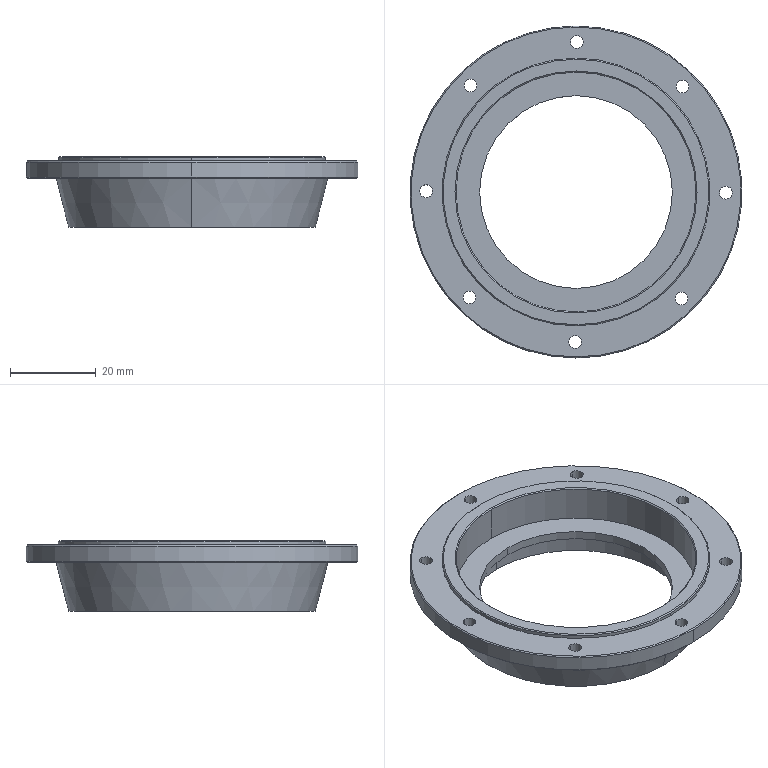Part | STEP file | 2026.6.15-Main Assembly图.sldasm-Part-83 | 1 solid | 42 faces | box 77.5 x 77.5 x 16.5 mm | volume 17666 mm3 | cylinder 26 | cone 10 | plane 6 | commonest cylinder face diameters 3 x16 45 x2 52.5 x2 56 x2 62.5 x2 77.5 x2
STEP:
#1=CARTESIAN_POINT('',(-1571.075,1457.755,3627.571));
#2=VERTEX_POINT('',#1);
#3=CARTESIAN_POINT('',(-1571.073,1460.755,3627.571));
#4=VERTEX_POINT('',#3);
#5=CARTESIAN_POINT('',(-1571.074,1459.255,3627.571));
#6=DIRECTION('',(0.,0.,-1.));
#7=DIRECTION('',(0.0007664,1.,0.));
#8=AXIS2_PLACEMENT_3D('',#5,#6,#7);
#9=CIRCLE('',#8,1.5);
#10=EDGE_CURVE('',#2,#4,#9,.T.);
#11=ORIENTED_EDGE('',*,*,#10,.T.);
#12=CARTESIAN_POINT('',(-1571.073,1460.755,3631.571));
#13=VERTEX_POINT('',#12);
#14=CARTESIAN_POINT('',(-1571.073,1460.755,3625.571));
#15=DIRECTION('',(0.,0.,1.));
#16=VECTOR('',#15,1000.);
#17=LINE('',#14,#16);
#18=EDGE_CURVE('',#4,#13,#17,.T.);
#19=ORIENTED_EDGE('',*,*,#18,.T.);
#20=CARTESIAN_POINT('',(-1571.075,1457.755,3631.571));
#21=VERTEX_POINT('',#20);
#22=CARTESIAN_POINT('',(-1571.074,1459.255,3631.571));
#23=DIRECTION('',(0.,0.,1.));
#24=DIRECTION('',(-0.7107,-0.7035,0.));
#25=AXIS2_PLACEMENT_3D('',#22,#23,#24);
#26=CIRCLE('',#25,1.5);
#27=EDGE_CURVE('',#13,#21,#26,.T.);
#28=ORIENTED_EDGE('',*,*,#27,.T.);
#29=CARTESIAN_POINT('',(-1571.075,1457.755,3625.571));
#30=DIRECTION('',(0.,0.,1.));
#31=VECTOR('',#30,1000.);
#32=LINE('',#29,#31);
#33=EDGE_CURVE('',#2,#21,#32,.T.);
#34=ORIENTED_EDGE('',*,*,#33,.F.);
#35=EDGE_LOOP('',(#11,#19,#28,#34));
#36=FACE_OUTER_BOUND('',#35,.T.);
#37=CARTESIAN_POINT('',(-1571.074,1459.255,3625.571));
#38=DIRECTION('',(0.,0.,1.));
#39=DIRECTION('',(-0.0007664,-1.,0.));
#40=AXIS2_PLACEMENT_3D('',#37,#38,#39);
#41=CYLINDRICAL_SURFACE('',#40,1.5);
#42=ADVANCED_FACE('',(#36),#41,.F.);
#43=CARTESIAN_POINT('',(-1595.876,1447.631,3627.571));
#44=VERTEX_POINT('',#43);
#45=CARTESIAN_POINT('',(-1595.874,1450.631,3627.571));
#46=VERTEX_POINT('',#45);
#47=CARTESIAN_POINT('',(-1595.875,1449.131,3627.571));
#48=DIRECTION('',(0.,0.,-1.));
#49=DIRECTION('',(0.0007664,1.,0.));
#50=AXIS2_PLACEMENT_3D('',#47,#48,#49);
#51=CIRCLE('',#50,1.5);
#52=EDGE_CURVE('',#44,#46,#51,.T.);
#53=ORIENTED_EDGE('',*,*,#52,.T.);
#54=CARTESIAN_POINT('',(-1595.874,1450.631,3631.571));
#55=VERTEX_POINT('',#54);
#56=CARTESIAN_POINT('',(-1595.874,1450.631,3625.571));
#57=DIRECTION('',(0.,0.,1.));
#58=VECTOR('',#57,1000.);
#59=LINE('',#56,#58);
#60=EDGE_CURVE('',#46,#55,#59,.T.);
#61=ORIENTED_EDGE('',*,*,#60,.T.);
#62=CARTESIAN_POINT('',(-1595.876,1447.631,3631.571));
#63=VERTEX_POINT('',#62);
#64=CARTESIAN_POINT('',(-1595.875,1449.131,3631.571));
#65=DIRECTION('',(0.,0.,1.));
#66=DIRECTION('',(-0.7107,-0.7035,0.));
#67=AXIS2_PLACEMENT_3D('',#64,#65,#66);
#68=CIRCLE('',#67,1.5);
#69=EDGE_CURVE('',#55,#63,#68,.T.);
#70=ORIENTED_EDGE('',*,*,#69,.T.);
#71=CARTESIAN_POINT('',(-1595.876,1447.631,3625.571));
#72=DIRECTION('',(0.,0.,1.));
#73=VECTOR('',#72,1000.);
#74=LINE('',#71,#73);
#75=EDGE_CURVE('',#44,#63,#74,.T.);
#76=ORIENTED_EDGE('',*,*,#75,.F.);
#77=EDGE_LOOP('',(#53,#61,#70,#76));
#78=FACE_OUTER_BOUND('',#77,.T.);
#79=CARTESIAN_POINT('',(-1595.875,1449.131,3625.571));
#80=DIRECTION('',(0.,0.,1.));
#81=DIRECTION('',(-0.0007664,-1.,0.));
#82=AXIS2_PLACEMENT_3D('',#79,#80,#81);
#83=CYLINDRICAL_SURFACE('',#82,1.5);
#84=ADVANCED_FACE('',(#78),#83,.F.);
#85=CARTESIAN_POINT('',(-1546.379,1447.378,3627.571));
#86=VERTEX_POINT('',#85);
#87=CARTESIAN_POINT('',(-1546.377,1450.378,3627.571));
#88=VERTEX_POINT('',#87);
#89=CARTESIAN_POINT('',(-1546.378,1448.878,3627.571));
#90=DIRECTION('',(0.,0.,-1.));
#91=DIRECTION('',(0.0007664,1.,0.));
#92=AXIS2_PLACEMENT_3D('',#89,#90,#91);
#93=CIRCLE('',#92,1.5);
#94=EDGE_CURVE('',#86,#88,#93,.T.);
#95=ORIENTED_EDGE('',*,*,#94,.T.);
#96=CARTESIAN_POINT('',(-1546.377,1450.378,3631.571));
#97=VERTEX_POINT('',#96);
#98=CARTESIAN_POINT('',(-1546.377,1450.378,3625.571));
#99=DIRECTION('',(0.,0.,1.));
#100=VECTOR('',#99,1000.);
#101=LINE('',#98,#100);
#102=EDGE_CURVE('',#88,#97,#101,.T.);
#103=ORIENTED_EDGE('',*,*,#102,.T.);
#104=CARTESIAN_POINT('',(-1546.379,1447.378,3631.571));
#105=VERTEX_POINT('',#104);
#106=CARTESIAN_POINT('',(-1546.378,1448.878,3631.571));
#107=DIRECTION('',(0.,0.,1.));
#108=DIRECTION('',(-0.7107,-0.7035,0.));
#109=AXIS2_PLACEMENT_3D('',#106,#107,#108);
#110=CIRCLE('',#109,1.5);
#111=EDGE_CURVE('',#97,#105,#110,.T.);
#112=ORIENTED_EDGE('',*,*,#111,.T.);
#113=CARTESIAN_POINT('',(-1546.379,1447.378,3625.571));
#114=DIRECTION('',(0.,0.,1.));
#115=VECTOR('',#114,1000.);
#116=LINE('',#113,#115);
#117=EDGE_CURVE('',#86,#105,#116,.T.);
#118=ORIENTED_EDGE('',*,*,#117,.F.);
#119=EDGE_LOOP('',(#95,#103,#112,#118));
#120=FACE_OUTER_BOUND('',#119,.T.);
#121=CARTESIAN_POINT('',(-1546.378,1448.878,3625.571));
#122=DIRECTION('',(0.,0.,1.));
#123=DIRECTION('',(-0.0007664,-1.,0.));
#124=AXIS2_PLACEMENT_3D('',#121,#122,#123);
#125=CYLINDRICAL_SURFACE('',#124,1.5);
#126=ADVANCED_FACE('',(#120),#125,.F.);
#127=CARTESIAN_POINT('',(-1606.254,1422.935,3627.571));
#128=VERTEX_POINT('',#127);
#129=CARTESIAN_POINT('',(-1606.252,1425.935,3627.571));
#130=VERTEX_POINT('',#129);
#131=CARTESIAN_POINT('',(-1606.253,1424.435,3627.571));
#132=DIRECTION('',(0.,0.,-1.));
#133=DIRECTION('',(0.0007664,1.,0.));
#134=AXIS2_PLACEMENT_3D('',#131,#132,#133);
#135=CIRCLE('',#134,1.5);
#136=EDGE_CURVE('',#128,#130,#135,.T.);
#137=ORIENTED_EDGE('',*,*,#136,.T.);
#138=CARTESIAN_POINT('',(-1606.252,1425.935,3631.571));
#139=VERTEX_POINT('',#138);
#140=CARTESIAN_POINT('',(-1606.252,1425.935,3625.571));
#141=DIRECTION('',(0.,0.,1.));
#142=VECTOR('',#141,1000.);
#143=LINE('',#140,#142);
#144=EDGE_CURVE('',#130,#139,#143,.T.);
#145=ORIENTED_EDGE('',*,*,#144,.T.);
#146=CARTESIAN_POINT('',(-1606.254,1422.935,3631.571));
#147=VERTEX_POINT('',#146);
#148=CARTESIAN_POINT('',(-1606.253,1424.435,3631.571));
#149=DIRECTION('',(0.,0.,1.));
#150=DIRECTION('',(-0.7107,-0.7035,0.));
#151=AXIS2_PLACEMENT_3D('',#148,#149,#150);
#152=CIRCLE('',#151,1.5);
#153=EDGE_CURVE('',#139,#147,#152,.T.);
#154=ORIENTED_EDGE('',*,*,#153,.T.);
#155=CARTESIAN_POINT('',(-1606.254,1422.935,3625.571));
#156=DIRECTION('',(0.,0.,1.));
#157=VECTOR('',#156,1000.);
#158=LINE('',#155,#157);
#159=EDGE_CURVE('',#128,#147,#158,.T.);
#160=ORIENTED_EDGE('',*,*,#159,.F.);
#161=EDGE_LOOP('',(#137,#145,#154,#160));
#162=FACE_OUTER_BOUND('',#161,.T.);
#163=CARTESIAN_POINT('',(-1606.253,1424.435,3625.571));
#164=DIRECTION('',(0.,0.,1.));
#165=DIRECTION('',(-0.0007664,-1.,0.));
#166=AXIS2_PLACEMENT_3D('',#163,#164,#165);
#167=CYLINDRICAL_SURFACE('',#166,1.5);
#168=ADVANCED_FACE('',(#162),#167,.F.);
#169=CARTESIAN_POINT('',(-1536.255,1422.577,3627.571));
#170=VERTEX_POINT('',#169);
#171=CARTESIAN_POINT('',(-1536.252,1425.577,3627.571));
#172=VERTEX_POINT('',#171);
#173=CARTESIAN_POINT('',(-1536.254,1424.077,3627.571));
#174=DIRECTION('',(0.,0.,-1.));
#175=DIRECTION('',(0.0007664,1.,0.));
#176=AXIS2_PLACEMENT_3D('',#173,#174,#175);
#177=CIRCLE('',#176,1.5);
#178=EDGE_CURVE('',#170,#172,#177,.T.);
#179=ORIENTED_EDGE('',*,*,#178,.T.);
#180=CARTESIAN_POINT('',(-1536.252,1425.577,3631.571));
#181=VERTEX_POINT('',#180);
#182=CARTESIAN_POINT('',(-1536.252,1425.577,3625.571));
#183=DIRECTION('',(0.,0.,1.));
#184=VECTOR('',#183,1000.);
#185=LINE('',#182,#184);
#186=EDGE_CURVE('',#172,#181,#185,.T.);
#187=ORIENTED_EDGE('',*,*,#186,.T.);
#188=CARTESIAN_POINT('',(-1536.255,1422.577,3631.571));
#189=VERTEX_POINT('',#188);
#190=CARTESIAN_POINT('',(-1536.254,1424.077,3631.571));
#191=DIRECTION('',(0.,0.,1.));
#192=DIRECTION('',(-0.7107,-0.7035,0.));
#193=AXIS2_PLACEMENT_3D('',#190,#191,#192);
#194=CIRCLE('',#193,1.5);
#195=EDGE_CURVE('',#181,#189,#194,.T.);
#196=ORIENTED_EDGE('',*,*,#195,.T.);
#197=CARTESIAN_POINT('',(-1536.255,1422.577,3625.571));
#198=DIRECTION('',(0.,0.,1.));
#199=VECTOR('',#198,1000.);
#200=LINE('',#197,#199);
#201=EDGE_CURVE('',#170,#189,#200,.T.);
#202=ORIENTED_EDGE('',*,*,#201,.F.);
#203=EDGE_LOOP('',(#179,#187,#196,#202));
#204=FACE_OUTER_BOUND('',#203,.T.);
#205=CARTESIAN_POINT('',(-1536.254,1424.077,3625.571));
#206=DIRECTION('',(0.,0.,1.));
#207=DIRECTION('',(-0.0007664,-1.,0.));
#208=AXIS2_PLACEMENT_3D('',#205,#206,#207);
#209=CYLINDRICAL_SURFACE('',#208,1.5);
#210=ADVANCED_FACE('',(#204),#209,.F.);
#211=CARTESIAN_POINT('',(-1596.129,1398.134,3627.571));
#212=VERTEX_POINT('',#211);
#213=CARTESIAN_POINT('',(-1596.127,1401.134,3627.571));
#214=VERTEX_POINT('',#213);
#215=CARTESIAN_POINT('',(-1596.128,1399.634,3627.571));
#216=DIRECTION('',(0.,0.,-1.));
#217=DIRECTION('',(0.0007664,1.,0.));
#218=AXIS2_PLACEMENT_3D('',#215,#216,#217);
#219=CIRCLE('',#218,1.5);
#220=EDGE_CURVE('',#212,#214,#219,.T.);
#221=ORIENTED_EDGE('',*,*,#220,.T.);
#222=CARTESIAN_POINT('',(-1596.127,1401.134,3631.571));
#223=VERTEX_POINT('',#222);
#224=CARTESIAN_POINT('',(-1596.127,1401.134,3625.571));
#225=DIRECTION('',(0.,0.,1.));
#226=VECTOR('',#225,1000.);
#227=LINE('',#224,#226);
#228=EDGE_CURVE('',#214,#223,#227,.T.);
#229=ORIENTED_EDGE('',*,*,#228,.T.);
#230=CARTESIAN_POINT('',(-1596.129,1398.134,3631.571));
#231=VERTEX_POINT('',#230);
#232=CARTESIAN_POINT('',(-1596.128,1399.634,3631.571));
#233=DIRECTION('',(0.,0.,1.));
#234=DIRECTION('',(-0.7107,-0.7035,0.));
#235=AXIS2_PLACEMENT_3D('',#232,#233,#234);
#236=CIRCLE('',#235,1.5);
#237=EDGE_CURVE('',#223,#231,#236,.T.);
#238=ORIENTED_EDGE('',*,*,#237,.T.);
#239=CARTESIAN_POINT('',(-1596.129,1398.134,3625.571));
#240=DIRECTION('',(0.,0.,1.));
#241=VECTOR('',#240,1000.);
#242=LINE('',#239,#241);
#243=EDGE_CURVE('',#212,#231,#242,.T.);
#244=ORIENTED_EDGE('',*,*,#243,.F.);
#245=EDGE_LOOP('',(#221,#229,#238,#244));
#246=FACE_OUTER_BOUND('',#245,.T.);
#247=CARTESIAN_POINT('',(-1596.128,1399.634,3625.571));
#248=DIRECTION('',(0.,0.,1.));
#249=DIRECTION('',(-0.0007664,-1.,0.));
#250=AXIS2_PLACEMENT_3D('',#247,#248,#249);
#251=CYLINDRICAL_SURFACE('',#250,1.5);
#252=ADVANCED_FACE('',(#246),#251,.F.);
#253=CARTESIAN_POINT('',(-1546.632,1397.881,3627.571));
#254=VERTEX_POINT('',#253);
#255=CARTESIAN_POINT('',(-1546.63,1400.881,3627.571));
#256=VERTEX_POINT('',#255);
#257=CARTESIAN_POINT('',(-1546.631,1399.381,3627.571));
#258=DIRECTION('',(0.,0.,-1.));
#259=DIRECTION('',(0.0007664,1.,0.));
#260=AXIS2_PLACEMENT_3D('',#257,#258,#259);
#261=CIRCLE('',#260,1.5);
#262=EDGE_CURVE('',#254,#256,#261,.T.);
#263=ORIENTED_EDGE('',*,*,#262,.T.);
#264=CARTESIAN_POINT('',(-1546.63,1400.881,3631.571));
#265=VERTEX_POINT('',#264);
#266=CARTESIAN_POINT('',(-1546.63,1400.881,3625.571));
#267=DIRECTION('',(0.,0.,1.));
#268=VECTOR('',#267,1000.);
#269=LINE('',#266,#268);
#270=EDGE_CURVE('',#256,#265,#269,.T.);
#271=ORIENTED_EDGE('',*,*,#270,.T.);
#272=CARTESIAN_POINT('',(-1546.632,1397.881,3631.571));
#273=VERTEX_POINT('',#272);
#274=CARTESIAN_POINT('',(-1546.631,1399.381,3631.571));
#275=DIRECTION('',(0.,0.,1.));
#276=DIRECTION('',(-0.7107,-0.7035,0.));
#277=AXIS2_PLACEMENT_3D('',#274,#275,#276);
#278=CIRCLE('',#277,1.5);
#279=EDGE_CURVE('',#265,#273,#278,.T.);
#280=ORIENTED_EDGE('',*,*,#279,.T.);
#281=CARTESIAN_POINT('',(-1546.632,1397.881,3625.571));
#282=DIRECTION('',(0.,0.,1.));
#283=VECTOR('',#282,1000.);
#284=LINE('',#281,#283);
#285=EDGE_CURVE('',#254,#273,#284,.T.);
#286=ORIENTED_EDGE('',*,*,#285,.F.);
#287=EDGE_LOOP('',(#263,#271,#280,#286));
#288=FACE_OUTER_BOUND('',#287,.T.);
#289=CARTESIAN_POINT('',(-1546.631,1399.381,3625.571));
#290=DIRECTION('',(0.,0.,1.));
#291=DIRECTION('',(-0.0007664,-1.,0.));
#292=AXIS2_PLACEMENT_3D('',#289,#290,#291);
#293=CYLINDRICAL_SURFACE('',#292,1.5);
#294=ADVANCED_FACE('',(#288),#293,.F.);
#295=CARTESIAN_POINT('',(-1571.433,1387.756,3627.571));
#296=VERTEX_POINT('',#295);
#297=CARTESIAN_POINT('',(-1571.431,1390.756,3627.571));
#298=VERTEX_POINT('',#297);
#299=CARTESIAN_POINT('',(-1571.432,1389.256,3627.571));
#300=DIRECTION('',(0.,0.,-1.));
#301=DIRECTION('',(0.0007664,1.,0.));
#302=AXIS2_PLACEMENT_3D('',#299,#300,#301);
#303=CIRCLE('',#302,1.5);
#304=EDGE_CURVE('',#296,#298,#303,.T.);
#305=ORIENTED_EDGE('',*,*,#304,.T.);
#306=CARTESIAN_POINT('',(-1571.431,1390.756,3631.571));
#307=VERTEX_POINT('',#306);
#308=CARTESIAN_POINT('',(-1571.431,1390.756,3625.571));
#309=DIRECTION('',(0.,0.,1.));
#310=VECTOR('',#309,1000.);
#311=LINE('',#308,#310);
#312=EDGE_CURVE('',#298,#307,#311,.T.);
#313=ORIENTED_EDGE('',*,*,#312,.T.);
#314=CARTESIAN_POINT('',(-1571.433,1387.756,3631.571));
#315=VERTEX_POINT('',#314);
#316=CARTESIAN_POINT('',(-1571.432,1389.256,3631.571));
#317=DIRECTION('',(0.,0.,1.));
#318=DIRECTION('',(-0.7107,-0.7035,0.));
#319=AXIS2_PLACEMENT_3D('',#316,#317,#318);
#320=CIRCLE('',#319,1.5);
#321=EDGE_CURVE('',#307,#315,#320,.T.);
#322=ORIENTED_EDGE('',*,*,#321,.T.);
#323=CARTESIAN_POINT('',(-1571.433,1387.756,3625.571));
#324=DIRECTION('',(0.,0.,1.));
#325=VECTOR('',#324,1000.);
#326=LINE('',#323,#325);
#327=EDGE_CURVE('',#296,#315,#326,.T.);
#328=ORIENTED_EDGE('',*,*,#327,.F.);
#329=EDGE_LOOP('',(#305,#313,#322,#328));
#330=FACE_OUTER_BOUND('',#329,.T.);
#331=CARTESIAN_POINT('',(-1571.432,1389.256,3625.571));
#332=DIRECTION('',(0.,0.,1.));
#333=DIRECTION('',(-0.0007664,-1.,0.));
#334=AXIS2_PLACEMENT_3D('',#331,#332,#333);
#335=CYLINDRICAL_SURFACE('',#334,1.5);
#336=ADVANCED_FACE('',(#330),#335,.F.);
#337=CARTESIAN_POINT('',(-1571.273,1398.006,3622.071));
#338=VERTEX_POINT('',#337);
#339=CARTESIAN_POINT('',(-1571.233,1450.506,3622.071));
#340=VERTEX_POINT('',#339);
#341=CARTESIAN_POINT('',(-1571.253,1424.256,3622.071));
#342=DIRECTION('',(0.,0.,-1.));
#343=DIRECTION('',(0.0007664,1.,0.));
#344=AXIS2_PLACEMENT_3D('',#341,#342,#343);
#345=CIRCLE('',#344,26.25);
#346=EDGE_CURVE('',#338,#340,#345,.T.);
#347=ORIENTED_EDGE('',*,*,#346,.F.);
#348=CARTESIAN_POINT('',(-1571.273,1398.006,3616.071));
#349=VERTEX_POINT('',#348);
#350=CARTESIAN_POINT('',(-1571.273,1398.006,3632.571));
#351=DIRECTION('',(0.,0.,-1.));
#352=VECTOR('',#351,1000.);
#353=LINE('',#350,#352);
#354=EDGE_CURVE('',#338,#349,#353,.T.);
#355=ORIENTED_EDGE('',*,*,#354,.T.);
#356=CARTESIAN_POINT('',(-1571.233,1450.506,3616.071));
#357=VERTEX_POINT('',#356);
#358=CARTESIAN_POINT('',(-1571.253,1424.256,3616.071));
#359=DIRECTION('',(0.,0.,-1.));
#360=DIRECTION('',(0.0007664,1.,0.));
#361=AXIS2_PLACEMENT_3D('',#358,#359,#360);
#362=CIRCLE('',#361,26.25);
#363=EDGE_CURVE('',#349,#357,#362,.T.);
#364=ORIENTED_EDGE('',*,*,#363,.T.);
#365=CARTESIAN_POINT('',(-1571.233,1450.506,3632.571));
#366=DIRECTION('',(0.,0.,-1.));
#367=VECTOR('',#366,1000.);
#368=LINE('',#365,#367);
#369=EDGE_CURVE('',#340,#357,#368,.T.);
#370=ORIENTED_EDGE('',*,*,#369,.F.);
#371=EDGE_LOOP('',(#347,#355,#364,#370));
#372=FACE_OUTER_BOUND('',#371,.T.);
#373=CARTESIAN_POINT('',(-1571.253,1424.256,3632.571));
#374=DIRECTION('',(0.,0.,-1.));
#375=DIRECTION('',(0.0007664,1.,0.));
#376=AXIS2_PLACEMENT_3D('',#373,#374,#375);
#377=CYLINDRICAL_SURFACE('',#376,26.25);
#378=ADVANCED_FACE('',(#372),#377,.F.);
#379=CARTESIAN_POINT('',(-1571.27,1401.756,3624.071));
#380=VERTEX_POINT('',#379);
#381=CARTESIAN_POINT('',(-1571.236,1446.756,3624.071));
#382=VERTEX_POINT('',#381);
#383=CARTESIAN_POINT('',(-1571.253,1424.256,3624.071));
#384=DIRECTION('',(0.,0.,-1.));
#385=DIRECTION('',(0.0007664,1.,0.));
#386=AXIS2_PLACEMENT_3D('',#383,#384,#385);
#387=CIRCLE('',#386,22.5);
#388=EDGE_CURVE('',#380,#382,#387,.T.);
#389=ORIENTED_EDGE('',*,*,#388,.F.);
#390=CARTESIAN_POINT('',(-1571.27,1401.756,3622.071));
#391=VERTEX_POINT('',#390);
#392=CARTESIAN_POINT('',(-1571.27,1401.756,3632.571));
#393=DIRECTION('',(0.,0.,-1.));
#394=VECTOR('',#393,1000.);
#395=LINE('',#392,#394);
#396=EDGE_CURVE('',#380,#391,#395,.T.);
#397=ORIENTED_EDGE('',*,*,#396,.T.);
#398=CARTESIAN_POINT('',(-1571.236,1446.756,3622.071));
#399=VERTEX_POINT('',#398);
#400=CARTESIAN_POINT('',(-1571.253,1424.256,3622.071));
#401=DIRECTION('',(0.,0.,-1.));
#402=DIRECTION('',(0.0007664,1.,0.));
#403=AXIS2_PLACEMENT_3D('',#400,#401,#402);
#404=CIRCLE('',#403,22.5);
#405=EDGE_CURVE('',#391,#399,#404,.T.);
#406=ORIENTED_EDGE('',*,*,#405,.T.);
#407=CARTESIAN_POINT('',(-1571.236,1446.756,3632.571));
#408=DIRECTION('',(0.,0.,-1.));
#409=VECTOR('',#408,1000.);
#410=LINE('',#407,#409);
#411=EDGE_CURVE('',#382,#399,#410,.T.);
#412=ORIENTED_EDGE('',*,*,#411,.F.);
#413=EDGE_LOOP('',(#389,#397,#406,#412));
#414=FACE_OUTER_BOUND('',#413,.T.);
#415=CARTESIAN_POINT('',(-1571.253,1424.256,3632.571));
#416=DIRECTION('',(0.,0.,-1.));
#417=DIRECTION('',(0.0007664,1.,0.));
#418=AXIS2_PLACEMENT_3D('',#415,#416,#417);
#419=CYLINDRICAL_SURFACE('',#418,22.5);
#420=ADVANCED_FACE('',(#414),#419,.F.);
#421=CARTESIAN_POINT('',(-1571.275,1396.256,3632.321));
#422=VERTEX_POINT('',#421);
#423=CARTESIAN_POINT('',(-1571.232,1452.256,3632.321));
#424=VERTEX_POINT('',#423);
#425=CARTESIAN_POINT('',(-1571.253,1424.256,3632.321));
#426=DIRECTION('',(0.,0.,-1.));
#427=DIRECTION('',(0.0007664,1.,0.));
#428=AXIS2_PLACEMENT_3D('',#425,#426,#427);
#429=CIRCLE('',#428,28.);
#430=EDGE_CURVE('',#422,#424,#429,.T.);
#431=ORIENTED_EDGE('',*,*,#430,.F.);
#432=CARTESIAN_POINT('',(-1571.275,1396.256,3624.071));
#433=VERTEX_POINT('',#432);
#434=CARTESIAN_POINT('',(-1571.275,1396.256,3632.571));
#435=DIRECTION('',(0.,0.,-1.));
#436=VECTOR('',#435,1000.);
#437=LINE('',#434,#436);
#438=EDGE_CURVE('',#422,#433,#437,.T.);
#439=ORIENTED_EDGE('',*,*,#438,.T.);
#440=CARTESIAN_POINT('',(-1571.232,1452.256,3624.071));
#441=VERTEX_POINT('',#440);
#442=CARTESIAN_POINT('',(-1571.253,1424.256,3624.071));
#443=DIRECTION('',(0.,0.,-1.));
#444=DIRECTION('',(0.0007664,1.,0.));
#445=AXIS2_PLACEMENT_3D('',#442,#443,#444);
#446=CIRCLE('',#445,28.);
#447=EDGE_CURVE('',#433,#441,#446,.T.);
#448=ORIENTED_EDGE('',*,*,#447,.T.);
#449=CARTESIAN_POINT('',(-1571.232,1452.256,3632.571));
#450=DIRECTION('',(0.,0.,-1.));
#451=VECTOR('',#450,1000.);
#452=LINE('',#449,#451);
#453=EDGE_CURVE('',#424,#441,#452,.T.);
#454=ORIENTED_EDGE('',*,*,#453,.F.);
#455=EDGE_LOOP('',(#431,#439,#448,#454));
#456=FACE_OUTER_BOUND('',#455,.T.);
#457=CARTESIAN_POINT('',(-1571.253,1424.256,3632.571));
#458=DIRECTION('',(0.,0.,-1.));
#459=DIRECTION('',(0.0007664,1.,0.));
#460=AXIS2_PLACEMENT_3D('',#457,#458,#459);
#461=CYLINDRICAL_SURFACE('',#460,28.);
#462=ADVANCED_FACE('',(#456),#461,.F.);
#463=ORIENTED_EDGE('',*,*,#430,.T.);
#464=CARTESIAN_POINT('',(-1571.231,1452.506,3632.571));
#465=VERTEX_POINT('',#464);
#466=CARTESIAN_POINT('',(-1571.231,1452.506,3632.571));
#467=DIRECTION('',(0.000542,0.7071,0.7071));
#468=VECTOR('',#467,1000.);
#469=LINE('',#466,#468);
#470=EDGE_CURVE('',#424,#465,#469,.T.);
#471=ORIENTED_EDGE('',*,*,#470,.T.);
#472=CARTESIAN_POINT('',(-1571.275,1396.006,3632.571));
#473=VERTEX_POINT('',#472);
#474=CARTESIAN_POINT('',(-1571.253,1424.256,3632.571));
#475=DIRECTION('',(0.,0.,-1.));
#476=DIRECTION('',(0.0007664,1.,0.));
#477=AXIS2_PLACEMENT_3D('',#474,#475,#476);
#478=CIRCLE('',#477,28.25);
#479=EDGE_CURVE('',#473,#465,#478,.T.);
#480=ORIENTED_EDGE('',*,*,#479,.F.);
#481=CARTESIAN_POINT('',(-1571.275,1396.006,3632.571));
#482=DIRECTION('',(-0.000542,-0.7071,0.7071));
#483=VECTOR('',#482,1000.);
#484=LINE('',#481,#483);
#485=EDGE_CURVE('',#422,#473,#484,.T.);
#486=ORIENTED_EDGE('',*,*,#485,.F.);
#487=EDGE_LOOP('',(#463,#471,#480,#486));
#488=FACE_OUTER_BOUND('',#487,.T.);
#489=CARTESIAN_POINT('',(-1571.253,1424.256,3632.571));
#490=DIRECTION('',(0.,0.,1.));
#491=DIRECTION('',(-0.0007664,-1.,0.));
#492=AXIS2_PLACEMENT_3D('',#489,#490,#491);
#493=CONICAL_SURFACE('',#492,28.25,0.7854);
#494=ADVANCED_FACE('',(#488),#493,.F.);
#495=CARTESIAN_POINT('',(-1571.229,1455.256,3632.571));
#496=VERTEX_POINT('',#495);
#497=CARTESIAN_POINT('',(-1571.277,1393.256,3632.571));
#498=VERTEX_POINT('',#497);
#499=CARTESIAN_POINT('',(-1571.253,1424.256,3632.571));
#500=DIRECTION('',(0.,0.,-1.));
#501=DIRECTION('',(0.0007664,1.,0.));
#502=AXIS2_PLACEMENT_3D('',#499,#500,#501);
#503=CIRCLE('',#502,31.);
#504=EDGE_CURVE('',#496,#498,#503,.T.);
#505=ORIENTED_EDGE('',*,*,#504,.T.);
#506=CARTESIAN_POINT('',(-1571.277,1393.006,3632.321));
#507=VERTEX_POINT('',#506);
#508=CARTESIAN_POINT('',(-1571.277,1393.006,3632.321));
#509=DIRECTION('',(-0.000542,-0.7071,-0.7071));
#510=VECTOR('',#509,1000.);
#511=LINE('',#508,#510);
#512=EDGE_CURVE('',#498,#507,#511,.T.);
#513=ORIENTED_EDGE('',*,*,#512,.T.);
#514=CARTESIAN_POINT('',(-1571.229,1455.506,3632.321));
#515=VERTEX_POINT('',#514);
#516=CARTESIAN_POINT('',(-1571.253,1424.256,3632.321));
#517=DIRECTION('',(0.,0.,-1.));
#518=DIRECTION('',(0.0007664,1.,0.));
#519=AXIS2_PLACEMENT_3D('',#516,#517,#518);
#520=CIRCLE('',#519,31.25);
#521=EDGE_CURVE('',#515,#507,#520,.T.);
#522=ORIENTED_EDGE('',*,*,#521,.F.);
#523=CARTESIAN_POINT('',(-1571.229,1455.506,3632.321));
#524=DIRECTION('',(0.000542,0.7071,-0.7071));
#525=VECTOR('',#524,1000.);
#526=LINE('',#523,#525);
#527=EDGE_CURVE('',#496,#515,#526,.T.);
#528=ORIENTED_EDGE('',*,*,#527,.F.);
#529=EDGE_LOOP('',(#505,#513,#522,#528));
#530=FACE_OUTER_BOUND('',#529,.T.);
#531=CARTESIAN_POINT('',(-1571.253,1424.256,3632.321));
#532=DIRECTION('',(0.,0.,-1.));
#533=DIRECTION('',(0.0007664,1.,0.));
#534=AXIS2_PLACEMENT_3D('',#531,#532,#533);
#535=CONICAL_SURFACE('',#534,31.25,0.7854);
#536=ADVANCED_FACE('',(#530),#535,.T.);
#537=ORIENTED_EDGE('',*,*,#521,.T.);
#538=CARTESIAN_POINT('',(-1571.277,1393.006,3631.571));
#539=VERTEX_POINT('',#538);
#540=CARTESIAN_POINT('',(-1571.277,1393.006,3632.571));
#541=DIRECTION('',(0.,0.,-1.));
#542=VECTOR('',#541,1000.);
#543=LINE('',#540,#542);
#544=EDGE_CURVE('',#507,#539,#543,.T.);
#545=ORIENTED_EDGE('',*,*,#544,.T.);
#546=CARTESIAN_POINT('',(-1571.229,1455.506,3631.571));
#547=VERTEX_POINT('',#546);
#548=CARTESIAN_POINT('',(-1571.253,1424.256,3631.571));
#549=DIRECTION('',(0.,0.,-1.));
#550=DIRECTION('',(0.0007664,1.,0.));
#551=AXIS2_PLACEMENT_3D('',#548,#549,#550);
#552=CIRCLE('',#551,31.25);
#553=EDGE_CURVE('',#547,#539,#552,.T.);
#554=ORIENTED_EDGE('',*,*,#553,.F.);
#555=CARTESIAN_POINT('',(-1571.229,1455.506,3632.571));
#556=DIRECTION('',(0.,0.,-1.));
#557=VECTOR('',#556,1000.);
#558=LINE('',#555,#557);
#559=EDGE_CURVE('',#515,#547,#558,.T.);
#560=ORIENTED_EDGE('',*,*,#559,.F.);
#561=EDGE_LOOP('',(#537,#545,#554,#560));
#562=FACE_OUTER_BOUND('',#561,.T.);
#563=CARTESIAN_POINT('',(-1571.253,1424.256,3632.571));
#564=DIRECTION('',(0.,0.,-1.));
#565=DIRECTION('',(0.0007664,1.,0.));
#566=AXIS2_PLACEMENT_3D('',#563,#564,#565);
#567=CYLINDRICAL_SURFACE('',#566,31.25);
#568=ADVANCED_FACE('',(#562),#567,.T.);
#569=CARTESIAN_POINT('',(-1571.224,1462.756,3631.571));
#570=VERTEX_POINT('',#569);
#571=CARTESIAN_POINT('',(-1571.283,1385.756,3631.571));
#572=VERTEX_POINT('',#571);
#573=CARTESIAN_POINT('',(-1571.253,1424.256,3631.571));
#574=DIRECTION('',(0.,0.,-1.));
#575=DIRECTION('',(0.0007664,1.,0.));
#576=AXIS2_PLACEMENT_3D('',#573,#574,#575);
#577=CIRCLE('',#576,38.5);
#578=EDGE_CURVE('',#570,#572,#577,.T.);
#579=ORIENTED_EDGE('',*,*,#578,.T.);
#580=CARTESIAN_POINT('',(-1571.283,1385.506,3631.321));
#581=VERTEX_POINT('',#580);
#582=CARTESIAN_POINT('',(-1571.283,1385.506,3631.321));
#583=DIRECTION('',(-0.000542,-0.7071,-0.7071));
#584=VECTOR('',#583,1000.);
#585=LINE('',#582,#584);
#586=EDGE_CURVE('',#572,#581,#585,.T.);
#587=ORIENTED_EDGE('',*,*,#586,.T.);
#588=CARTESIAN_POINT('',(-1571.223,1463.006,3631.321));
#589=VERTEX_POINT('',#588);
#590=CARTESIAN_POINT('',(-1571.253,1424.256,3631.321));
#591=DIRECTION('',(0.,0.,-1.));
#592=DIRECTION('',(0.0007664,1.,0.));
#593=AXIS2_PLACEMENT_3D('',#590,#591,#592);
#594=CIRCLE('',#593,38.75);
#595=EDGE_CURVE('',#589,#581,#594,.T.);
#596=ORIENTED_EDGE('',*,*,#595,.F.);
#597=CARTESIAN_POINT('',(-1571.223,1463.006,3631.321));
#598=DIRECTION('',(0.000542,0.7071,-0.7071));
#599=VECTOR('',#598,1000.);
#600=LINE('',#597,#599);
#601=EDGE_CURVE('',#570,#589,#600,.T.);
#602=ORIENTED_EDGE('',*,*,#601,.F.);
#603=EDGE_LOOP('',(#579,#587,#596,#602));
#604=FACE_OUTER_BOUND('',#603,.T.);
#605=CARTESIAN_POINT('',(-1571.253,1424.256,3631.321));
#606=DIRECTION('',(0.,0.,-1.));
#607=DIRECTION('',(0.0007664,1.,0.));
#608=AXIS2_PLACEMENT_3D('',#605,#606,#607);
#609=CONICAL_SURFACE('',#608,38.75,0.7854);
#610=ADVANCED_FACE('',(#604),#609,.T.);
#611=ORIENTED_EDGE('',*,*,#595,.T.);
#612=CARTESIAN_POINT('',(-1571.283,1385.506,3627.821));
#613=VERTEX_POINT('',#612);
#614=CARTESIAN_POINT('',(-1571.283,1385.506,3632.571));
#615=DIRECTION('',(0.,0.,-1.));
#616=VECTOR('',#615,1000.);
#617=LINE('',#614,#616);
#618=EDGE_CURVE('',#581,#613,#617,.T.);
#619=ORIENTED_EDGE('',*,*,#618,.T.);
#620=CARTESIAN_POINT('',(-1571.223,1463.006,3627.821));
#621=VERTEX_POINT('',#620);
#622=CARTESIAN_POINT('',(-1571.253,1424.256,3627.821));
#623=DIRECTION('',(0.,0.,-1.));
#624=DIRECTION('',(0.0007664,1.,0.));
#625=AXIS2_PLACEMENT_3D('',#622,#623,#624);
#626=CIRCLE('',#625,38.75);
#627=EDGE_CURVE('',#621,#613,#626,.T.);
#628=ORIENTED_EDGE('',*,*,#627,.F.);
#629=CARTESIAN_POINT('',(-1571.223,1463.006,3632.571));
#630=DIRECTION('',(0.,0.,-1.));
#631=VECTOR('',#630,1000.);
#632=LINE('',#629,#631);
#633=EDGE_CURVE('',#589,#621,#632,.T.);
#634=ORIENTED_EDGE('',*,*,#633,.F.);
#635=EDGE_LOOP('',(#611,#619,#628,#634));
#636=FACE_OUTER_BOUND('',#635,.T.);
#637=CARTESIAN_POINT('',(-1571.253,1424.256,3632.571));
#638=DIRECTION('',(0.,0.,-1.));
#639=DIRECTION('',(0.0007664,1.,0.));
#640=AXIS2_PLACEMENT_3D('',#637,#638,#639);
#641=CYLINDRICAL_SURFACE('',#640,38.75);
#642=ADVANCED_FACE('',(#636),#641,.T.);
#643=CARTESIAN_POINT('',(-1571.224,1462.756,3627.571));
#644=VERTEX_POINT('',#643);
#645=CARTESIAN_POINT('',(-1571.283,1385.756,3627.571));
#646=VERTEX_POINT('',#645);
#647=CARTESIAN_POINT('',(-1571.253,1424.256,3627.571));
#648=DIRECTION('',(0.,0.,-1.));
#649=DIRECTION('',(0.0007664,1.,0.));
#650=AXIS2_PLACEMENT_3D('',#647,#648,#649);
#651=CIRCLE('',#650,38.5);
#652=EDGE_CURVE('',#644,#646,#651,.T.);
#653=ORIENTED_EDGE('',*,*,#652,.F.);
#654=CARTESIAN_POINT('',(-1571.224,1462.756,3627.571));
#655=DIRECTION('',(0.000542,0.7071,0.7071));
#656=VECTOR('',#655,1000.);
#657=LINE('',#654,#656);
#658=EDGE_CURVE('',#644,#621,#657,.T.);
#659=ORIENTED_EDGE('',*,*,#658,.T.);
#660=ORIENTED_EDGE('',*,*,#627,.T.);
#661=CARTESIAN_POINT('',(-1571.283,1385.756,3627.571));
#662=DIRECTION('',(-0.000542,-0.7071,0.7071));
#663=VECTOR('',#662,1000.);
#664=LINE('',#661,#663);
#665=EDGE_CURVE('',#646,#613,#664,.T.);
#666=ORIENTED_EDGE('',*,*,#665,.F.);
#667=EDGE_LOOP('',(#653,#659,#660,#666));
#668=FACE_OUTER_BOUND('',#667,.T.);
#669=CARTESIAN_POINT('',(-1571.253,1424.256,3627.571));
#670=DIRECTION('',(0.,0.,1.));
#671=DIRECTION('',(-0.0007664,-1.,0.));
#672=AXIS2_PLACEMENT_3D('',#669,#670,#671);
#673=CONICAL_SURFACE('',#672,38.5,0.7854);
#674=ADVANCED_FACE('',(#668),#673,.T.);
#675=CARTESIAN_POINT('',(-1571.231,1453.006,3616.071));
#676=VERTEX_POINT('',#675);
#677=CARTESIAN_POINT('',(-1571.275,1395.506,3616.071));
#678=VERTEX_POINT('',#677);
#679=CARTESIAN_POINT('',(-1571.253,1424.256,3616.071));
#680=DIRECTION('',(0.,0.,-1.));
#681=DIRECTION('',(0.0007664,1.,0.));
#682=AXIS2_PLACEMENT_3D('',#679,#680,#681);
#683=CIRCLE('',#682,28.75);
#684=EDGE_CURVE('',#676,#678,#683,.T.);
#685=ORIENTED_EDGE('',*,*,#684,.F.);
#686=CARTESIAN_POINT('',(-1571.229,1456.006,3627.571));
#687=VERTEX_POINT('',#686);
#688=CARTESIAN_POINT('',(-1571.231,1453.006,3616.071));
#689=DIRECTION('',(0.0001935,0.2524,0.9676));
#690=VECTOR('',#689,1000.);
#691=LINE('',#688,#690);
#692=EDGE_CURVE('',#676,#687,#691,.T.);
#693=ORIENTED_EDGE('',*,*,#692,.T.);
#694=CARTESIAN_POINT('',(-1571.277,1392.506,3627.571));
#695=VERTEX_POINT('',#694);
#696=CARTESIAN_POINT('',(-1571.253,1424.256,3627.571));
#697=DIRECTION('',(0.,0.,-1.));
#698=DIRECTION('',(0.0007664,1.,0.));
#699=AXIS2_PLACEMENT_3D('',#696,#697,#698);
#700=CIRCLE('',#699,31.75);
#701=EDGE_CURVE('',#687,#695,#700,.T.);
#702=ORIENTED_EDGE('',*,*,#701,.T.);
#703=CARTESIAN_POINT('',(-1571.275,1395.506,3616.071));
#704=DIRECTION('',(-0.0001935,-0.2524,0.9676));
#705=VECTOR('',#704,1000.);
#706=LINE('',#703,#705);
#707=EDGE_CURVE('',#678,#695,#706,.T.);
#708=ORIENTED_EDGE('',*,*,#707,.F.);
#709=EDGE_LOOP('',(#685,#693,#702,#708));
#710=FACE_OUTER_BOUND('',#709,.T.);
#711=CARTESIAN_POINT('',(-1571.253,1424.256,3616.071));
#712=DIRECTION('',(0.,0.,1.));
#713=DIRECTION('',(-0.0007664,-1.,0.));
#714=AXIS2_PLACEMENT_3D('',#711,#712,#713);
#715=CONICAL_SURFACE('',#714,28.75,0.2552);
#716=ADVANCED_FACE('',(#710),#715,.T.);
#717=CARTESIAN_POINT('',(-1571.253,1424.256,3616.071));
#718=DIRECTION('',(0.,0.,-1.));
#719=DIRECTION('',(0.0007664,1.,0.));
#720=AXIS2_PLACEMENT_3D('',#717,#718,#719);
#721=CIRCLE('',#720,28.75);
#722=EDGE_CURVE('',#678,#676,#721,.T.);
#723=ORIENTED_EDGE('',*,*,#722,.T.);
#724=ORIENTED_EDGE('',*,*,#684,.T.);
#725=EDGE_LOOP('',(#723,#724));
#726=FACE_OUTER_BOUND('',#725,.T.);
#727=CARTESIAN_POINT('',(-1571.253,1424.256,3616.071));
#728=DIRECTION('',(0.,0.,-1.));
#729=DIRECTION('',(0.0007664,1.,0.));
#730=AXIS2_PLACEMENT_3D('',#727,#728,#729);
#731=CIRCLE('',#730,26.25);
#732=EDGE_CURVE('',#357,#349,#731,.T.);
#733=ORIENTED_EDGE('',*,*,#732,.F.);
#734=ORIENTED_EDGE('',*,*,#363,.F.);
#735=EDGE_LOOP('',(#733,#734));
#736=FACE_BOUND('',#735,.T.);
#737=CARTESIAN_POINT('',(-1589.909,1405.789,3616.071));
#738=DIRECTION('',(0.,0.,-1.));
#739=DIRECTION('',(0.0007664,1.,0.));
#740=AXIS2_PLACEMENT_3D('',#737,#738,#739);
#741=PLANE('',#740);
#742=ADVANCED_FACE('',(#726,#736),#741,.T.);
#743=ORIENTED_EDGE('',*,*,#692,.F.);
#744=ORIENTED_EDGE('',*,*,#722,.F.);
#745=ORIENTED_EDGE('',*,*,#707,.T.);
#746=CARTESIAN_POINT('',(-1571.253,1424.256,3627.571));
#747=DIRECTION('',(0.,0.,-1.));
#748=DIRECTION('',(0.0007664,1.,0.));
#749=AXIS2_PLACEMENT_3D('',#746,#747,#748);
#750=CIRCLE('',#749,31.75);
#751=EDGE_CURVE('',#695,#687,#750,.T.);
#752=ORIENTED_EDGE('',*,*,#751,.T.);
#753=EDGE_LOOP('',(#743,#744,#745,#752));
#754=FACE_OUTER_BOUND('',#753,.T.);
#755=CARTESIAN_POINT('',(-1571.253,1424.256,3616.071));
#756=DIRECTION('',(0.,0.,1.));
#757=DIRECTION('',(-0.0007664,-1.,0.));
#758=AXIS2_PLACEMENT_3D('',#755,#756,#757);
#759=CONICAL_SURFACE('',#758,28.75,0.2552);
#760=ADVANCED_FACE('',(#754),#759,.T.);
#761=ORIENTED_EDGE('',*,*,#10,.F.);
#762=CARTESIAN_POINT('',(-1571.074,1459.255,3627.571));
#763=DIRECTION('',(0.,0.,-1.));
#764=DIRECTION('',(0.0007664,1.,0.));
#765=AXIS2_PLACEMENT_3D('',#762,#763,#764);
#766=CIRCLE('',#765,1.5);
#767=EDGE_CURVE('',#4,#2,#766,.T.);
#768=ORIENTED_EDGE('',*,*,#767,.F.);
#769=EDGE_LOOP('',(#761,#768));
#770=FACE_BOUND('',#769,.T.);
#771=ORIENTED_EDGE('',*,*,#52,.F.);
#772=CARTESIAN_POINT('',(-1595.875,1449.131,3627.571));
#773=DIRECTION('',(0.,0.,-1.));
#774=DIRECTION('',(0.0007664,1.,0.));
#775=AXIS2_PLACEMENT_3D('',#772,#773,#774);
#776=CIRCLE('',#775,1.5);
#777=EDGE_CURVE('',#46,#44,#776,.T.);
#778=ORIENTED_EDGE('',*,*,#777,.F.);
#779=EDGE_LOOP('',(#771,#778));
#780=FACE_BOUND('',#779,.T.);
#781=ORIENTED_EDGE('',*,*,#94,.F.);
#782=CARTESIAN_POINT('',(-1546.378,1448.878,3627.571));
#783=DIRECTION('',(0.,0.,-1.));
#784=DIRECTION('',(0.0007664,1.,0.));
#785=AXIS2_PLACEMENT_3D('',#782,#783,#784);
#786=CIRCLE('',#785,1.5);
#787=EDGE_CURVE('',#88,#86,#786,.T.);
#788=ORIENTED_EDGE('',*,*,#787,.F.);
#789=EDGE_LOOP('',(#781,#788));
#790=FACE_BOUND('',#789,.T.);
#791=ORIENTED_EDGE('',*,*,#136,.F.);
#792=CARTESIAN_POINT('',(-1606.253,1424.435,3627.571));
#793=DIRECTION('',(0.,0.,-1.));
#794=DIRECTION('',(0.0007664,1.,0.));
#795=AXIS2_PLACEMENT_3D('',#792,#793,#794);
#796=CIRCLE('',#795,1.5);
#797=EDGE_CURVE('',#130,#128,#796,.T.);
#798=ORIENTED_EDGE('',*,*,#797,.F.);
#799=EDGE_LOOP('',(#791,#798));
#800=FACE_BOUND('',#799,.T.);
#801=ORIENTED_EDGE('',*,*,#178,.F.);
#802=CARTESIAN_POINT('',(-1536.254,1424.077,3627.571));
#803=DIRECTION('',(0.,0.,-1.));
#804=DIRECTION('',(0.0007664,1.,0.));
#805=AXIS2_PLACEMENT_3D('',#802,#803,#804);
#806=CIRCLE('',#805,1.5);
#807=EDGE_CURVE('',#172,#170,#806,.T.);
#808=ORIENTED_EDGE('',*,*,#807,.F.);
#809=EDGE_LOOP('',(#801,#808));
#810=FACE_BOUND('',#809,.T.);
#811=ORIENTED_EDGE('',*,*,#220,.F.);
#812=CARTESIAN_POINT('',(-1596.128,1399.634,3627.571));
#813=DIRECTION('',(0.,0.,-1.));
#814=DIRECTION('',(0.0007664,1.,0.));
#815=AXIS2_PLACEMENT_3D('',#812,#813,#814);
#816=CIRCLE('',#815,1.5);
#817=EDGE_CURVE('',#214,#212,#816,.T.);
#818=ORIENTED_EDGE('',*,*,#817,.F.);
#819=EDGE_LOOP('',(#811,#818));
#820=FACE_BOUND('',#819,.T.);
#821=ORIENTED_EDGE('',*,*,#262,.F.);
#822=CARTESIAN_POINT('',(-1546.631,1399.381,3627.571));
#823=DIRECTION('',(0.,0.,-1.));
#824=DIRECTION('',(0.0007664,1.,0.));
#825=AXIS2_PLACEMENT_3D('',#822,#823,#824);
#826=CIRCLE('',#825,1.5);
#827=EDGE_CURVE('',#256,#254,#826,.T.);
#828=ORIENTED_EDGE('',*,*,#827,.F.);
#829=EDGE_LOOP('',(#821,#828));
#830=FACE_BOUND('',#829,.T.);
#831=ORIENTED_EDGE('',*,*,#304,.F.);
#832=CARTESIAN_POINT('',(-1571.432,1389.256,3627.571));
#833=DIRECTION('',(0.,0.,-1.));
#834=DIRECTION('',(0.0007664,1.,0.));
#835=AXIS2_PLACEMENT_3D('',#832,#833,#834);
#836=CIRCLE('',#835,1.5);
#837=EDGE_CURVE('',#298,#296,#836,.T.);
#838=ORIENTED_EDGE('',*,*,#837,.F.);
#839=EDGE_LOOP('',(#831,#838));
#840=FACE_BOUND('',#839,.T.);
#841=CARTESIAN_POINT('',(-1571.253,1424.256,3627.571));
#842=DIRECTION('',(0.,0.,-1.));
#843=DIRECTION('',(0.0007664,1.,0.));
#844=AXIS2_PLACEMENT_3D('',#841,#842,#843);
#845=CIRCLE('',#844,38.5);
#846=EDGE_CURVE('',#646,#644,#845,.T.);
#847=ORIENTED_EDGE('',*,*,#846,.T.);
#848=ORIENTED_EDGE('',*,*,#652,.T.);
#849=EDGE_LOOP('',(#847,#848));
#850=FACE_OUTER_BOUND('',#849,.T.);
#851=ORIENTED_EDGE('',*,*,#751,.F.);
#852=ORIENTED_EDGE('',*,*,#701,.F.);
#853=EDGE_LOOP('',(#851,#852));
#854=FACE_BOUND('',#853,.T.);
#855=CARTESIAN_POINT('',(-1593.818,1401.92,3627.571));
#856=DIRECTION('',(0.,0.,-1.));
#857=DIRECTION('',(0.0007664,1.,0.));
#858=AXIS2_PLACEMENT_3D('',#855,#856,#857);
#859=PLANE('',#858);
#860=ADVANCED_FACE('',(#770,#780,#790,#800,#810,#820,#830,#840,#850,#854),#859,.T.);
#861=ORIENTED_EDGE('',*,*,#658,.F.);
#862=ORIENTED_EDGE('',*,*,#846,.F.);
#863=ORIENTED_EDGE('',*,*,#665,.T.);
#864=CARTESIAN_POINT('',(-1571.253,1424.256,3627.821));
#865=DIRECTION('',(0.,0.,-1.));
#866=DIRECTION('',(0.0007664,1.,0.));
#867=AXIS2_PLACEMENT_3D('',#864,#865,#866);
#868=CIRCLE('',#867,38.75);
#869=EDGE_CURVE('',#613,#621,#868,.T.);
#870=ORIENTED_EDGE('',*,*,#869,.T.);
#871=EDGE_LOOP('',(#861,#862,#863,#870));
#872=FACE_OUTER_BOUND('',#871,.T.);
#873=CARTESIAN_POINT('',(-1571.253,1424.256,3627.571));
#874=DIRECTION('',(0.,0.,1.));
#875=DIRECTION('',(-0.0007664,-1.,0.));
#876=AXIS2_PLACEMENT_3D('',#873,#874,#875);
#877=CONICAL_SURFACE('',#876,38.5,0.7854);
#878=ADVANCED_FACE('',(#872),#877,.T.);
#879=ORIENTED_EDGE('',*,*,#618,.F.);
#880=CARTESIAN_POINT('',(-1571.253,1424.256,3631.321));
#881=DIRECTION('',(0.,0.,-1.));
#882=DIRECTION('',(0.0007664,1.,0.));
#883=AXIS2_PLACEMENT_3D('',#880,#881,#882);
#884=CIRCLE('',#883,38.75);
#885=EDGE_CURVE('',#581,#589,#884,.T.);
#886=ORIENTED_EDGE('',*,*,#885,.T.);
#887=ORIENTED_EDGE('',*,*,#633,.T.);
#888=ORIENTED_EDGE('',*,*,#869,.F.);
#889=EDGE_LOOP('',(#879,#886,#887,#888));
#890=FACE_OUTER_BOUND('',#889,.T.);
#891=CARTESIAN_POINT('',(-1571.253,1424.256,3632.571));
#892=DIRECTION('',(0.,0.,-1.));
#893=DIRECTION('',(0.0007664,1.,0.));
#894=AXIS2_PLACEMENT_3D('',#891,#892,#893);
#895=CYLINDRICAL_SURFACE('',#894,38.75);
#896=ADVANCED_FACE('',(#890),#895,.T.);
#897=ORIENTED_EDGE('',*,*,#586,.F.);
#898=CARTESIAN_POINT('',(-1571.253,1424.256,3631.571));
#899=DIRECTION('',(0.,0.,-1.));
#900=DIRECTION('',(0.0007664,1.,0.));
#901=AXIS2_PLACEMENT_3D('',#898,#899,#900);
#902=CIRCLE('',#901,38.5);
#903=EDGE_CURVE('',#572,#570,#902,.T.);
#904=ORIENTED_EDGE('',*,*,#903,.T.);
#905=ORIENTED_EDGE('',*,*,#601,.T.);
#906=ORIENTED_EDGE('',*,*,#885,.F.);
#907=EDGE_LOOP('',(#897,#904,#905,#906));
#908=FACE_OUTER_BOUND('',#907,.T.);
#909=CARTESIAN_POINT('',(-1571.253,1424.256,3631.321));
#910=DIRECTION('',(0.,0.,-1.));
#911=DIRECTION('',(0.0007664,1.,0.));
#912=AXIS2_PLACEMENT_3D('',#909,#910,#911);
#913=CONICAL_SURFACE('',#912,38.75,0.7854);
#914=ADVANCED_FACE('',(#908),#913,.T.);
#915=CARTESIAN_POINT('',(-1571.074,1459.255,3631.571));
#916=DIRECTION('',(0.,0.,1.));
#917=DIRECTION('',(-0.7107,-0.7035,0.));
#918=AXIS2_PLACEMENT_3D('',#915,#916,#917);
#919=CIRCLE('',#918,1.5);
#920=EDGE_CURVE('',#21,#13,#919,.T.);
#921=ORIENTED_EDGE('',*,*,#920,.F.);
#922=ORIENTED_EDGE('',*,*,#27,.F.);
#923=EDGE_LOOP('',(#921,#922));
#924=FACE_BOUND('',#923,.T.);
#925=CARTESIAN_POINT('',(-1595.875,1449.131,3631.571));
#926=DIRECTION('',(0.,0.,1.));
#927=DIRECTION('',(-0.7107,-0.7035,0.));
#928=AXIS2_PLACEMENT_3D('',#925,#926,#927);
#929=CIRCLE('',#928,1.5);
#930=EDGE_CURVE('',#63,#55,#929,.T.);
#931=ORIENTED_EDGE('',*,*,#930,.F.);
#932=ORIENTED_EDGE('',*,*,#69,.F.);
#933=EDGE_LOOP('',(#931,#932));
#934=FACE_BOUND('',#933,.T.);
#935=CARTESIAN_POINT('',(-1546.378,1448.878,3631.571));
#936=DIRECTION('',(0.,0.,1.));
#937=DIRECTION('',(-0.7107,-0.7035,0.));
#938=AXIS2_PLACEMENT_3D('',#935,#936,#937);
#939=CIRCLE('',#938,1.5);
#940=EDGE_CURVE('',#105,#97,#939,.T.);
#941=ORIENTED_EDGE('',*,*,#940,.F.);
#942=ORIENTED_EDGE('',*,*,#111,.F.);
#943=EDGE_LOOP('',(#941,#942));
#944=FACE_BOUND('',#943,.T.);
#945=CARTESIAN_POINT('',(-1606.253,1424.435,3631.571));
#946=DIRECTION('',(0.,0.,1.));
#947=DIRECTION('',(-0.7107,-0.7035,0.));
#948=AXIS2_PLACEMENT_3D('',#945,#946,#947);
#949=CIRCLE('',#948,1.5);
#950=EDGE_CURVE('',#147,#139,#949,.T.);
#951=ORIENTED_EDGE('',*,*,#950,.F.);
#952=ORIENTED_EDGE('',*,*,#153,.F.);
#953=EDGE_LOOP('',(#951,#952));
#954=FACE_BOUND('',#953,.T.);
#955=CARTESIAN_POINT('',(-1536.254,1424.077,3631.571));
#956=DIRECTION('',(0.,0.,1.));
#957=DIRECTION('',(-0.7107,-0.7035,0.));
#958=AXIS2_PLACEMENT_3D('',#955,#956,#957);
#959=CIRCLE('',#958,1.5);
#960=EDGE_CURVE('',#189,#181,#959,.T.);
#961=ORIENTED_EDGE('',*,*,#960,.F.);
#962=ORIENTED_EDGE('',*,*,#195,.F.);
#963=EDGE_LOOP('',(#961,#962));
#964=FACE_BOUND('',#963,.T.);
#965=CARTESIAN_POINT('',(-1596.128,1399.634,3631.571));
#966=DIRECTION('',(0.,0.,1.));
#967=DIRECTION('',(-0.7107,-0.7035,0.));
#968=AXIS2_PLACEMENT_3D('',#965,#966,#967);
#969=CIRCLE('',#968,1.5);
#970=EDGE_CURVE('',#231,#223,#969,.T.);
#971=ORIENTED_EDGE('',*,*,#970,.F.);
#972=ORIENTED_EDGE('',*,*,#237,.F.);
#973=EDGE_LOOP('',(#971,#972));
#974=FACE_BOUND('',#973,.T.);
#975=CARTESIAN_POINT('',(-1546.631,1399.381,3631.571));
#976=DIRECTION('',(0.,0.,1.));
#977=DIRECTION('',(-0.7107,-0.7035,0.));
#978=AXIS2_PLACEMENT_3D('',#975,#976,#977);
#979=CIRCLE('',#978,1.5);
#980=EDGE_CURVE('',#273,#265,#979,.T.);
#981=ORIENTED_EDGE('',*,*,#980,.F.);
#982=ORIENTED_EDGE('',*,*,#279,.F.);
#983=EDGE_LOOP('',(#981,#982));
#984=FACE_BOUND('',#983,.T.);
#985=CARTESIAN_POINT('',(-1571.432,1389.256,3631.571));
#986=DIRECTION('',(0.,0.,1.));
#987=DIRECTION('',(-0.7107,-0.7035,0.));
#988=AXIS2_PLACEMENT_3D('',#985,#986,#987);
#989=CIRCLE('',#988,1.5);
#990=EDGE_CURVE('',#315,#307,#989,.T.);
#991=ORIENTED_EDGE('',*,*,#990,.F.);
#992=ORIENTED_EDGE('',*,*,#321,.F.);
#993=EDGE_LOOP('',(#991,#992));
#994=FACE_BOUND('',#993,.T.);
#995=ORIENTED_EDGE('',*,*,#553,.T.);
#996=CARTESIAN_POINT('',(-1571.253,1424.256,3631.571));
#997=DIRECTION('',(0.,0.,-1.));
#998=DIRECTION('',(0.0007664,1.,0.));
#999=AXIS2_PLACEMENT_3D('',#996,#997,#998);
#1000=CIRCLE('',#999,31.25);
#1001=EDGE_CURVE('',#539,#547,#1000,.T.);
#1002=ORIENTED_EDGE('',*,*,#1001,.T.);
#1003=EDGE_LOOP('',(#995,#1002));
#1004=FACE_BOUND('',#1003,.T.);
#1005=ORIENTED_EDGE('',*,*,#578,.F.);
#1006=ORIENTED_EDGE('',*,*,#903,.F.);
#1007=EDGE_LOOP('',(#1005,#1006));
#1008=FACE_OUTER_BOUND('',#1007,.T.);
#1009=CARTESIAN_POINT('',(-1598.616,1397.172,3631.571));
#1010=DIRECTION('',(0.,0.,1.));
#1011=DIRECTION('',(-0.0007664,-1.,0.));
#1012=AXIS2_PLACEMENT_3D('',#1009,#1010,#1011);
#1013=PLANE('',#1012);
#1014=ADVANCED_FACE('',(#924,#934,#944,#954,#964,#974,#984,#994,#1004,#1008),#1013,.T.);
#1015=ORIENTED_EDGE('',*,*,#544,.F.);
#1016=CARTESIAN_POINT('',(-1571.253,1424.256,3632.321));
#1017=DIRECTION('',(0.,0.,-1.));
#1018=DIRECTION('',(0.0007664,1.,0.));
#1019=AXIS2_PLACEMENT_3D('',#1016,#1017,#1018);
#1020=CIRCLE('',#1019,31.25);
#1021=EDGE_CURVE('',#507,#515,#1020,.T.);
#1022=ORIENTED_EDGE('',*,*,#1021,.T.);
#1023=ORIENTED_EDGE('',*,*,#559,.T.);
#1024=ORIENTED_EDGE('',*,*,#1001,.F.);
#1025=EDGE_LOOP('',(#1015,#1022,#1023,#1024));
#1026=FACE_OUTER_BOUND('',#1025,.T.);
#1027=CARTESIAN_POINT('',(-1571.253,1424.256,3632.571));
#1028=DIRECTION('',(0.,0.,-1.));
#1029=DIRECTION('',(0.0007664,1.,0.));
#1030=AXIS2_PLACEMENT_3D('',#1027,#1028,#1029);
#1031=CYLINDRICAL_SURFACE('',#1030,31.25);
#1032=ADVANCED_FACE('',(#1026),#1031,.T.);
#1033=ORIENTED_EDGE('',*,*,#512,.F.);
#1034=CARTESIAN_POINT('',(-1571.253,1424.256,3632.571));
#1035=DIRECTION('',(0.,0.,-1.));
#1036=DIRECTION('',(0.0007664,1.,0.));
#1037=AXIS2_PLACEMENT_3D('',#1034,#1035,#1036);
#1038=CIRCLE('',#1037,31.);
#1039=EDGE_CURVE('',#498,#496,#1038,.T.);
#1040=ORIENTED_EDGE('',*,*,#1039,.T.);
#1041=ORIENTED_EDGE('',*,*,#527,.T.);
#1042=ORIENTED_EDGE('',*,*,#1021,.F.);
#1043=EDGE_LOOP('',(#1033,#1040,#1041,#1042));
#1044=FACE_OUTER_BOUND('',#1043,.T.);
#1045=CARTESIAN_POINT('',(-1571.253,1424.256,3632.321));
#1046=DIRECTION('',(0.,0.,-1.));
#1047=DIRECTION('',(0.0007664,1.,0.));
#1048=AXIS2_PLACEMENT_3D('',#1045,#1046,#1047);
#1049=CONICAL_SURFACE('',#1048,31.25,0.7854);
#1050=ADVANCED_FACE('',(#1044),#1049,.T.);
#1051=ORIENTED_EDGE('',*,*,#479,.T.);
#1052=CARTESIAN_POINT('',(-1571.253,1424.256,3632.571));
#1053=DIRECTION('',(0.,0.,-1.));
#1054=DIRECTION('',(0.0007664,1.,0.));
#1055=AXIS2_PLACEMENT_3D('',#1052,#1053,#1054);
#1056=CIRCLE('',#1055,28.25);
#1057=EDGE_CURVE('',#465,#473,#1056,.T.);
#1058=ORIENTED_EDGE('',*,*,#1057,.T.);
#1059=EDGE_LOOP('',(#1051,#1058));
#1060=FACE_BOUND('',#1059,.T.);
#1061=ORIENTED_EDGE('',*,*,#504,.F.);
#1062=ORIENTED_EDGE('',*,*,#1039,.F.);
#1063=EDGE_LOOP('',(#1061,#1062));
#1064=FACE_OUTER_BOUND('',#1063,.T.);
#1065=CARTESIAN_POINT('',(-1593.285,1402.448,3632.571));
#1066=DIRECTION('',(0.,0.,1.));
#1067=DIRECTION('',(-0.0007664,-1.,0.));
#1068=AXIS2_PLACEMENT_3D('',#1065,#1066,#1067);
#1069=PLANE('',#1068);
#1070=ADVANCED_FACE('',(#1060,#1064),#1069,.T.);
#1071=ORIENTED_EDGE('',*,*,#470,.F.);
#1072=CARTESIAN_POINT('',(-1571.253,1424.256,3632.321));
#1073=DIRECTION('',(0.,0.,-1.));
#1074=DIRECTION('',(0.0007664,1.,0.));
#1075=AXIS2_PLACEMENT_3D('',#1072,#1073,#1074);
#1076=CIRCLE('',#1075,28.);
#1077=EDGE_CURVE('',#424,#422,#1076,.T.);
#1078=ORIENTED_EDGE('',*,*,#1077,.T.);
#1079=ORIENTED_EDGE('',*,*,#485,.T.);
#1080=ORIENTED_EDGE('',*,*,#1057,.F.);
#1081=EDGE_LOOP('',(#1071,#1078,#1079,#1080));
#1082=FACE_OUTER_BOUND('',#1081,.T.);
#1083=CARTESIAN_POINT('',(-1571.253,1424.256,3632.571));
#1084=DIRECTION('',(0.,0.,1.));
#1085=DIRECTION('',(-0.0007664,-1.,0.));
#1086=AXIS2_PLACEMENT_3D('',#1083,#1084,#1085);
#1087=CONICAL_SURFACE('',#1086,28.25,0.7854);
#1088=ADVANCED_FACE('',(#1082),#1087,.F.);
#1089=ORIENTED_EDGE('',*,*,#438,.F.);
#1090=ORIENTED_EDGE('',*,*,#1077,.F.);
#1091=ORIENTED_EDGE('',*,*,#453,.T.);
#1092=CARTESIAN_POINT('',(-1571.253,1424.256,3624.071));
#1093=DIRECTION('',(0.,0.,-1.));
#1094=DIRECTION('',(0.0007664,1.,0.));
#1095=AXIS2_PLACEMENT_3D('',#1092,#1093,#1094);
#1096=CIRCLE('',#1095,28.);
#1097=EDGE_CURVE('',#441,#433,#1096,.T.);
#1098=ORIENTED_EDGE('',*,*,#1097,.T.);
#1099=EDGE_LOOP('',(#1089,#1090,#1091,#1098));
#1100=FACE_OUTER_BOUND('',#1099,.T.);
#1101=CARTESIAN_POINT('',(-1571.253,1424.256,3632.571));
#1102=DIRECTION('',(0.,0.,-1.));
#1103=DIRECTION('',(0.0007664,1.,0.));
#1104=AXIS2_PLACEMENT_3D('',#1101,#1102,#1103);
#1105=CYLINDRICAL_SURFACE('',#1104,28.);
#1106=ADVANCED_FACE('',(#1100),#1105,.F.);
#1107=CARTESIAN_POINT('',(-1571.253,1424.256,3624.071));
#1108=DIRECTION('',(0.,0.,-1.));
#1109=DIRECTION('',(0.0007664,1.,0.));
#1110=AXIS2_PLACEMENT_3D('',#1107,#1108,#1109);
#1111=CIRCLE('',#1110,22.5);
#1112=EDGE_CURVE('',#382,#380,#1111,.T.);
#1113=ORIENTED_EDGE('',*,*,#1112,.T.);
#1114=ORIENTED_EDGE('',*,*,#388,.T.);
#1115=EDGE_LOOP('',(#1113,#1114));
#1116=FACE_BOUND('',#1115,.T.);
#1117=ORIENTED_EDGE('',*,*,#1097,.F.);
#1118=ORIENTED_EDGE('',*,*,#447,.F.);
#1119=EDGE_LOOP('',(#1117,#1118));
#1120=FACE_OUTER_BOUND('',#1119,.T.);
#1121=CARTESIAN_POINT('',(-1591.153,1404.558,3624.071));
#1122=DIRECTION('',(0.,0.,1.));
#1123=DIRECTION('',(-0.0007664,-1.,0.));
#1124=AXIS2_PLACEMENT_3D('',#1121,#1122,#1123);
#1125=PLANE('',#1124);
#1126=ADVANCED_FACE('',(#1116,#1120),#1125,.T.);
#1127=ORIENTED_EDGE('',*,*,#396,.F.);
#1128=ORIENTED_EDGE('',*,*,#1112,.F.);
#1129=ORIENTED_EDGE('',*,*,#411,.T.);
#1130=CARTESIAN_POINT('',(-1571.253,1424.256,3622.071));
#1131=DIRECTION('',(0.,0.,-1.));
#1132=DIRECTION('',(0.0007664,1.,0.));
#1133=AXIS2_PLACEMENT_3D('',#1130,#1131,#1132);
#1134=CIRCLE('',#1133,22.5);
#1135=EDGE_CURVE('',#399,#391,#1134,.T.);
#1136=ORIENTED_EDGE('',*,*,#1135,.T.);
#1137=EDGE_LOOP('',(#1127,#1128,#1129,#1136));
#1138=FACE_OUTER_BOUND('',#1137,.T.);
#1139=CARTESIAN_POINT('',(-1571.253,1424.256,3632.571));
#1140=DIRECTION('',(0.,0.,-1.));
#1141=DIRECTION('',(0.0007664,1.,0.));
#1142=AXIS2_PLACEMENT_3D('',#1139,#1140,#1141);
#1143=CYLINDRICAL_SURFACE('',#1142,22.5);
#1144=ADVANCED_FACE('',(#1138),#1143,.F.);
#1145=CARTESIAN_POINT('',(-1571.253,1424.256,3622.071));
#1146=DIRECTION('',(0.,0.,-1.));
#1147=DIRECTION('',(0.0007664,1.,0.));
#1148=AXIS2_PLACEMENT_3D('',#1145,#1146,#1147);
#1149=CIRCLE('',#1148,26.25);
#1150=EDGE_CURVE('',#340,#338,#1149,.T.);
#1151=ORIENTED_EDGE('',*,*,#1150,.T.);
#1152=ORIENTED_EDGE('',*,*,#346,.T.);
#1153=EDGE_LOOP('',(#1151,#1152));
#1154=FACE_OUTER_BOUND('',#1153,.T.);
#1155=ORIENTED_EDGE('',*,*,#1135,.F.);
#1156=ORIENTED_EDGE('',*,*,#405,.F.);
#1157=EDGE_LOOP('',(#1155,#1156));
#1158=FACE_BOUND('',#1157,.T.);
#1159=CARTESIAN_POINT('',(-1587.244,1408.428,3622.071));
#1160=DIRECTION('',(0.,0.,-1.));
#1161=DIRECTION('',(0.0007664,1.,0.));
#1162=AXIS2_PLACEMENT_3D('',#1159,#1160,#1161);
#1163=PLANE('',#1162);
#1164=ADVANCED_FACE('',(#1154,#1158),#1163,.T.);
#1165=ORIENTED_EDGE('',*,*,#354,.F.);
#1166=ORIENTED_EDGE('',*,*,#1150,.F.);
#1167=ORIENTED_EDGE('',*,*,#369,.T.);
#1168=ORIENTED_EDGE('',*,*,#732,.T.);
#1169=EDGE_LOOP('',(#1165,#1166,#1167,#1168));
#1170=FACE_OUTER_BOUND('',#1169,.T.);
#1171=CARTESIAN_POINT('',(-1571.253,1424.256,3632.571));
#1172=DIRECTION('',(0.,0.,-1.));
#1173=DIRECTION('',(0.0007664,1.,0.));
#1174=AXIS2_PLACEMENT_3D('',#1171,#1172,#1173);
#1175=CYLINDRICAL_SURFACE('',#1174,26.25);
#1176=ADVANCED_FACE('',(#1170),#1175,.F.);
#1177=ORIENTED_EDGE('',*,*,#312,.F.);
#1178=ORIENTED_EDGE('',*,*,#837,.T.);
#1179=ORIENTED_EDGE('',*,*,#327,.T.);
#1180=ORIENTED_EDGE('',*,*,#990,.T.);
#1181=EDGE_LOOP('',(#1177,#1178,#1179,#1180));
#1182=FACE_OUTER_BOUND('',#1181,.T.);
#1183=CARTESIAN_POINT('',(-1571.432,1389.256,3625.571));
#1184=DIRECTION('',(0.,0.,1.));
#1185=DIRECTION('',(-0.0007664,-1.,0.));
#1186=AXIS2_PLACEMENT_3D('',#1183,#1184,#1185);
#1187=CYLINDRICAL_SURFACE('',#1186,1.5);
#1188=ADVANCED_FACE('',(#1182),#1187,.F.);
#1189=ORIENTED_EDGE('',*,*,#270,.F.);
#1190=ORIENTED_EDGE('',*,*,#827,.T.);
#1191=ORIENTED_EDGE('',*,*,#285,.T.);
#1192=ORIENTED_EDGE('',*,*,#980,.T.);
#1193=EDGE_LOOP('',(#1189,#1190,#1191,#1192));
#1194=FACE_OUTER_BOUND('',#1193,.T.);
#1195=CARTESIAN_POINT('',(-1546.631,1399.381,3625.571));
#1196=DIRECTION('',(0.,0.,1.));
#1197=DIRECTION('',(-0.0007664,-1.,0.));
#1198=AXIS2_PLACEMENT_3D('',#1195,#1196,#1197);
#1199=CYLINDRICAL_SURFACE('',#1198,1.5);
#1200=ADVANCED_FACE('',(#1194),#1199,.F.);
#1201=ORIENTED_EDGE('',*,*,#228,.F.);
#1202=ORIENTED_EDGE('',*,*,#817,.T.);
#1203=ORIENTED_EDGE('',*,*,#243,.T.);
#1204=ORIENTED_EDGE('',*,*,#970,.T.);
#1205=EDGE_LOOP('',(#1201,#1202,#1203,#1204));
#1206=FACE_OUTER_BOUND('',#1205,.T.);
#1207=CARTESIAN_POINT('',(-1596.128,1399.634,3625.571));
#1208=DIRECTION('',(0.,0.,1.));
#1209=DIRECTION('',(-0.0007664,-1.,0.));
#1210=AXIS2_PLACEMENT_3D('',#1207,#1208,#1209);
#1211=CYLINDRICAL_SURFACE('',#1210,1.5);
#1212=ADVANCED_FACE('',(#1206),#1211,.F.);
#1213=ORIENTED_EDGE('',*,*,#186,.F.);
#1214=ORIENTED_EDGE('',*,*,#807,.T.);
#1215=ORIENTED_EDGE('',*,*,#201,.T.);
#1216=ORIENTED_EDGE('',*,*,#960,.T.);
#1217=EDGE_LOOP('',(#1213,#1214,#1215,#1216));
#1218=FACE_OUTER_BOUND('',#1217,.T.);
#1219=CARTESIAN_POINT('',(-1536.254,1424.077,3625.571));
#1220=DIRECTION('',(0.,0.,1.));
#1221=DIRECTION('',(-0.0007664,-1.,0.));
#1222=AXIS2_PLACEMENT_3D('',#1219,#1220,#1221);
#1223=CYLINDRICAL_SURFACE('',#1222,1.5);
#1224=ADVANCED_FACE('',(#1218),#1223,.F.);
#1225=ORIENTED_EDGE('',*,*,#144,.F.);
#1226=ORIENTED_EDGE('',*,*,#797,.T.);
#1227=ORIENTED_EDGE('',*,*,#159,.T.);
#1228=ORIENTED_EDGE('',*,*,#950,.T.);
#1229=EDGE_LOOP('',(#1225,#1226,#1227,#1228));
#1230=FACE_OUTER_BOUND('',#1229,.T.);
#1231=CARTESIAN_POINT('',(-1606.253,1424.435,3625.571));
#1232=DIRECTION('',(0.,0.,1.));
#1233=DIRECTION('',(-0.0007664,-1.,0.));
#1234=AXIS2_PLACEMENT_3D('',#1231,#1232,#1233);
#1235=CYLINDRICAL_SURFACE('',#1234,1.5);
#1236=ADVANCED_FACE('',(#1230),#1235,.F.);
#1237=ORIENTED_EDGE('',*,*,#102,.F.);
#1238=ORIENTED_EDGE('',*,*,#787,.T.);
#1239=ORIENTED_EDGE('',*,*,#117,.T.);
#1240=ORIENTED_EDGE('',*,*,#940,.T.);
#1241=EDGE_LOOP('',(#1237,#1238,#1239,#1240));
#1242=FACE_OUTER_BOUND('',#1241,.T.);
#1243=CARTESIAN_POINT('',(-1546.378,1448.878,3625.571));
#1244=DIRECTION('',(0.,0.,1.));
#1245=DIRECTION('',(-0.0007664,-1.,0.));
#1246=AXIS2_PLACEMENT_3D('',#1243,#1244,#1245);
#1247=CYLINDRICAL_SURFACE('',#1246,1.5);
#1248=ADVANCED_FACE('',(#1242),#1247,.F.);
#1249=ORIENTED_EDGE('',*,*,#60,.F.);
#1250=ORIENTED_EDGE('',*,*,#777,.T.);
#1251=ORIENTED_EDGE('',*,*,#75,.T.);
#1252=ORIENTED_EDGE('',*,*,#930,.T.);
#1253=EDGE_LOOP('',(#1249,#1250,#1251,#1252));
#1254=FACE_OUTER_BOUND('',#1253,.T.);
#1255=CARTESIAN_POINT('',(-1595.875,1449.131,3625.571));
#1256=DIRECTION('',(0.,0.,1.));
#1257=DIRECTION('',(-0.0007664,-1.,0.));
#1258=AXIS2_PLACEMENT_3D('',#1255,#1256,#1257);
#1259=CYLINDRICAL_SURFACE('',#1258,1.5);
#1260=ADVANCED_FACE('',(#1254),#1259,.F.);
#1261=ORIENTED_EDGE('',*,*,#18,.F.);
#1262=ORIENTED_EDGE('',*,*,#767,.T.);
#1263=ORIENTED_EDGE('',*,*,#33,.T.);
#1264=ORIENTED_EDGE('',*,*,#920,.T.);
#1265=EDGE_LOOP('',(#1261,#1262,#1263,#1264));
#1266=FACE_OUTER_BOUND('',#1265,.T.);
#1267=CARTESIAN_POINT('',(-1571.074,1459.255,3625.571));
#1268=DIRECTION('',(0.,0.,1.));
#1269=DIRECTION('',(-0.0007664,-1.,0.));
#1270=AXIS2_PLACEMENT_3D('',#1267,#1268,#1269);
#1271=CYLINDRICAL_SURFACE('',#1270,1.5);
#1272=ADVANCED_FACE('',(#1266),#1271,.F.);
#1273=CLOSED_SHELL('',(#42,#84,#126,#168,#210,#252,#294,#336,#378,#420,#462,#494,#536,#568,#610,#642,#674,#716,#742,#760,#860,#878,#896,#914,#1014,#1032,#1050,#1070,#1088,#1106,#1126,#1144,#1164,#1176,#1188,#1200,#1212,#1224,#1236,#1248,#1260,#1272));
#1274=MANIFOLD_SOLID_BREP('',#1273);
#1275=CARTESIAN_POINT('',(0.,0.,0.));
#1276=DIRECTION('',(0.,0.,1.));
#1277=DIRECTION('',(1.,0.,0.));
#1278=AXIS2_PLACEMENT_3D('',#1275,#1276,#1277);
#1279=(LENGTH_UNIT()NAMED_UNIT(*)SI_UNIT(.MILLI.,.METRE.));
#1280=UNCERTAINTY_MEASURE_WITH_UNIT(LENGTH_MEASURE(0.00001),#1279,'','');
#1281=(NAMED_UNIT(*)PLANE_ANGLE_UNIT()SI_UNIT($,.RADIAN.));
#1282=(NAMED_UNIT(*)SI_UNIT($,.STERADIAN.)SOLID_ANGLE_UNIT());
#1283=(GEOMETRIC_REPRESENTATION_CONTEXT(3)GLOBAL_UNCERTAINTY_ASSIGNED_CONTEXT((#1280))GLOBAL_UNIT_ASSIGNED_CONTEXT((#1279,#1281,#1282))REPRESENTATION_CONTEXT('',''));
#1284=ADVANCED_BREP_SHAPE_REPRESENTATION('',(#1274,#1278),#1283);